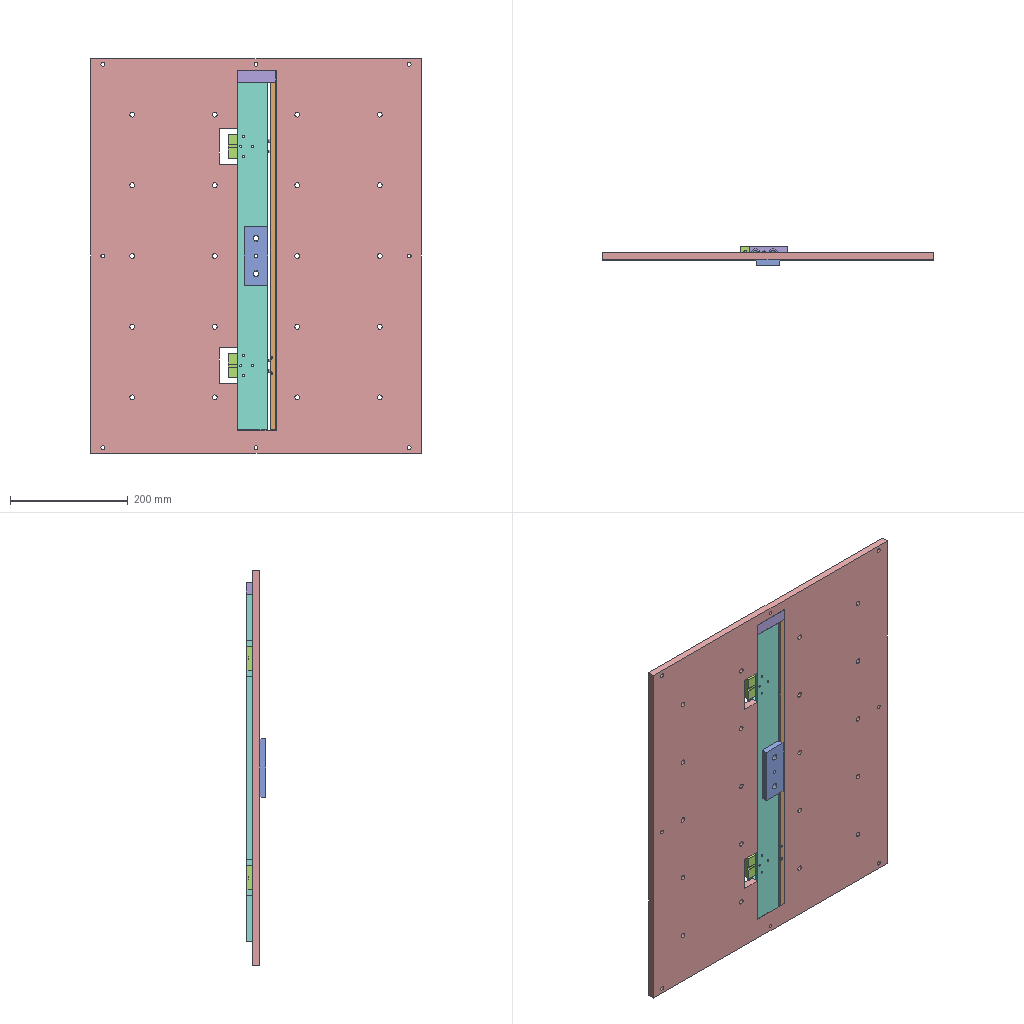Assembly | SolidWorks | 9 different items | 12 placed | box 560 x 33 x 670 mm
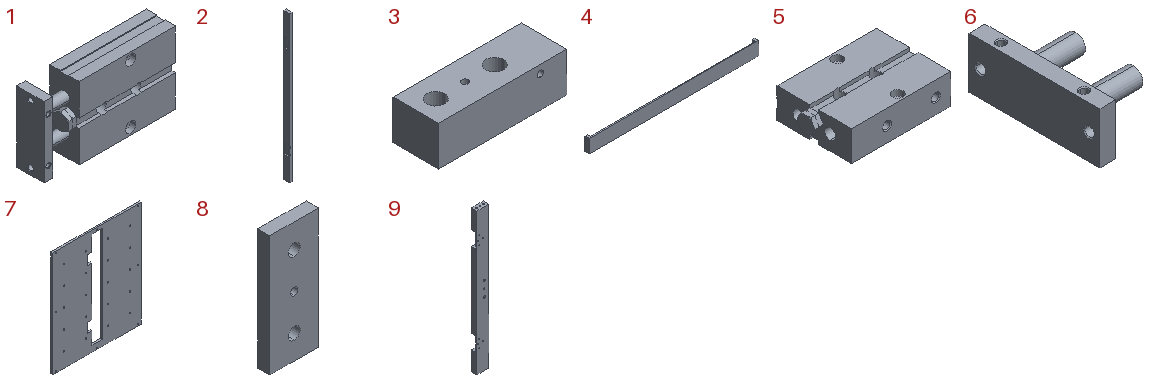Parts list (item | name | quantity | parent item | size | volume | features):
1 | (subassembly) | x2 | - | 75.8 x 17 x 42 mm | 41331 mm3 | -
2 | - | x1 | - | 10 x 23 x 590 mm | 128132 mm3 | features 3DProfileFeature 2, HoleWzd 2, MirrorPattern 2, Cut 1, Extrusion 1
3 | - | x1 | - | 64.8 x 23 x 20 mm | 24913 mm3 | features 3DProfileFeature 2, HoleWzd 2, Extrusion 1, ICE 1
4 | - | x1 | - | 670 x 16 x 52.685 mm | 357606 mm3 | features HoleWzd 2, MirrorPattern 2, Extrusion 1, Fillet 1, ICE 1
5 | - | x2 | in 1 | 60.8 x 42 x 17 mm | 37225 mm3 | features BaseBody 1
6 | - | x2 | in 1 | 22 x 41 x 16 mm | 4106 mm3 | features BaseBody 1
7 | - | x1 | - | 560 x 12 x 670 mm | 3956531 mm3 | features MirrorPattern 3, Cut 2, Extrusion 1, HoleWzd 1, ICE 1
8 | - | x1 | - | 40 x 10 x 100 mm | 38146 mm3 | features Extrusion 1
9 | - | x1 | - | 49.8 x 23 x 590 mm | 566573 mm3 | features 3DProfileFeature 4, HoleWzd 4, MirrorPattern 4, Cut 3, ICE 3, Extrusion 1
Mates (type | each side: item.copy, entity, surface, feature):
In the top assembly
Coincident | 7.1 face plane Boss-Extrude1 | 8.1 face plane Boss-Extrude1
Parallel | 7.1 face plane Boss-Extrude1 | 8.1 face plane Boss-Extrude1
Concentric | 8.1 face cylinder Boss-Extrude1 | 9.1 face cylinder CBORE for M8 Hex Socket Head Cap Screw0 | 2 times
Coincident | 8.1 face plane Boss-Extrude1 | 9.1 face plane Boss-Extrude1
DistanceDim | 5.1 face plane Imported1 | 9.1 face plane Boss-Extrude1
Coincident | 5.2 face plane Imported1 | 5.1 face plane Imported1
Parallel | 5.2 face plane Imported1 | 5.1 face plane Imported1
Coincident | 6.1 face plane Imported1 | 6.2 face plane Imported1
Coincident | 5.1 face plane Imported1 | 9.1 face plane Boss-Extrude4
Concentric | 5.1 face cylinder Imported1 | 9.1 face cylinder Cut-Extrude3
Concentric | 5.2 face cylinder Imported1 | 9.1 face cylinder Mirror4
Coincident | 9.1 face plane Boss-Extrude1 | 2.1 face plane Boss-Extrude1 | 2 times
Coincident | 6.2 face plane Imported1 | 2.1 face plane Boss-Extrude1
Concentric | 7.1 select_type:24 | 9.1 face cylinder CBORE for M5 Hex Head Bolt1
Parallel | 7.1 face plane Boss-Extrude1 | 9.1 face plane Boss-Extrude1
Coincident | 9.1 face plane Boss-Extrude1 | 3.1 face plane Boss-Extrude1 | 3 times
In subassembly 1
Concentric | 5.3 face cylinder Imported1 | 6.3 face cylinder Imported1 | 2 times
LimitDistanceDim | 6.3 face plane Imported1 | 5.3 face plane Imported1